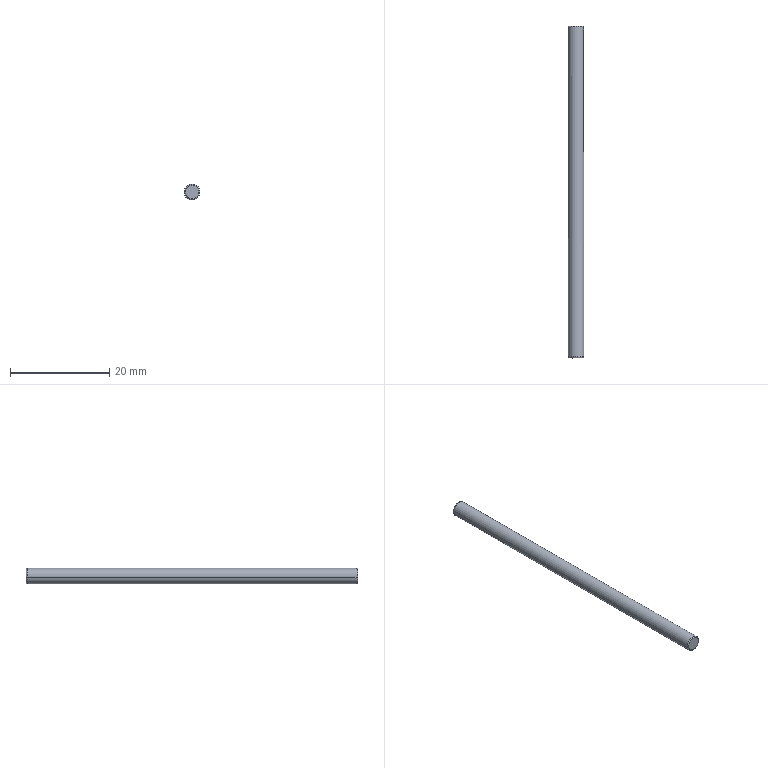Part | SolidWorks | features BaseBody 1 | 1 solid | 8 faces | box 3.204 x 67.003 x 3.14 mm | volume 518.664 mm3 | torus 4 | cylinder 2 | plane 2 | commonest cylinder face diameters 3.14 x2
STEP:
#1=CARTESIAN_POINT('',(340.446,372.663,106.551));
#2=VERTEX_POINT('',#1);
#3=CARTESIAN_POINT('',(343.498,372.666,107.288));
#4=VERTEX_POINT('',#3);
#5=CARTESIAN_POINT('',(341.972,372.664,106.919));
#6=DIRECTION('',(0.0009599,-1.,0.));
#7=DIRECTION('',(0.9721,0.0009331,0.2347));
#8=AXIS2_PLACEMENT_3D('',#5,#6,#7);
#9=CIRCLE('',#8,1.57);
#10=EDGE_CURVE('',#2,#4,#9,.T.);
#11=ORIENTED_EDGE('',*,*,#10,.T.);
#12=CARTESIAN_POINT('',(343.304,372.465,107.241));
#13=VERTEX_POINT('',#12);
#14=CARTESIAN_POINT('',(343.304,372.665,107.241));
#15=DIRECTION('',(0.2347,0.0002252,-0.9721));
#16=DIRECTION('',(-0.9721,0.,-0.2347));
#17=AXIS2_PLACEMENT_3D('',#14,#15,#16);
#18=CIRCLE('',#17,0.2);
#19=EDGE_CURVE('',#4,#13,#18,.T.);
#20=ORIENTED_EDGE('',*,*,#19,.T.);
#21=CARTESIAN_POINT('',(340.641,372.463,106.598));
#22=VERTEX_POINT('',#21);
#23=CARTESIAN_POINT('',(341.972,372.464,106.919));
#24=DIRECTION('',(0.0009599,-1.,0.));
#25=DIRECTION('',(0.9721,0.0009331,0.2347));
#26=AXIS2_PLACEMENT_3D('',#23,#24,#25);
#27=CIRCLE('',#26,1.37);
#28=EDGE_CURVE('',#22,#13,#27,.T.);
#29=ORIENTED_EDGE('',*,*,#28,.F.);
#30=CARTESIAN_POINT('',(340.64,372.663,106.598));
#31=DIRECTION('',(-0.2347,-0.0002252,0.9721));
#32=DIRECTION('',(0.9721,0.,0.2347));
#33=AXIS2_PLACEMENT_3D('',#30,#31,#32);
#34=CIRCLE('',#33,0.2);
#35=EDGE_CURVE('',#2,#22,#34,.T.);
#36=ORIENTED_EDGE('',*,*,#35,.F.);
#37=EDGE_LOOP('',(#11,#20,#29,#36));
#38=FACE_OUTER_BOUND('',#37,.T.);
#39=CARTESIAN_POINT('',(341.972,372.664,106.919));
#40=DIRECTION('',(0.0009599,-1.,0.));
#41=DIRECTION('',(-0.9721,-0.0009331,-0.2347));
#42=AXIS2_PLACEMENT_3D('',#39,#40,#41);
#43=TOROIDAL_SURFACE('',#42,1.37,0.2);
#44=ADVANCED_FACE('',(#38),#43,.T.);
#45=CARTESIAN_POINT('',(343.434,439.265,107.288));
#46=VERTEX_POINT('',#45);
#47=CARTESIAN_POINT('',(340.382,439.263,106.551));
#48=VERTEX_POINT('',#47);
#49=CARTESIAN_POINT('',(341.908,439.264,106.919));
#50=DIRECTION('',(-0.0009599,1.,0.));
#51=DIRECTION('',(0.9721,0.0009331,0.2347));
#52=AXIS2_PLACEMENT_3D('',#49,#50,#51);
#53=CIRCLE('',#52,1.57);
#54=EDGE_CURVE('',#46,#48,#53,.T.);
#55=ORIENTED_EDGE('',*,*,#54,.F.);
#56=CARTESIAN_POINT('',(343.434,439.465,107.288));
#57=DIRECTION('',(0.0009599,-1.,0.));
#58=VECTOR('',#57,1000.);
#59=LINE('',#56,#58);
#60=EDGE_CURVE('',#46,#4,#59,.T.);
#61=ORIENTED_EDGE('',*,*,#60,.T.);
#62=ORIENTED_EDGE('',*,*,#10,.F.);
#63=CARTESIAN_POINT('',(340.382,439.463,106.551));
#64=DIRECTION('',(0.0009599,-1.,0.));
#65=VECTOR('',#64,1000.);
#66=LINE('',#63,#65);
#67=EDGE_CURVE('',#48,#2,#66,.T.);
#68=ORIENTED_EDGE('',*,*,#67,.F.);
#69=EDGE_LOOP('',(#55,#61,#62,#68));
#70=FACE_OUTER_BOUND('',#69,.T.);
#71=CARTESIAN_POINT('',(341.908,439.464,106.919));
#72=DIRECTION('',(0.0009599,-1.,0.));
#73=DIRECTION('',(-0.9721,-0.0009331,-0.2347));
#74=AXIS2_PLACEMENT_3D('',#71,#72,#73);
#75=CYLINDRICAL_SURFACE('',#74,1.57);
#76=ADVANCED_FACE('',(#70),#75,.T.);
#77=CARTESIAN_POINT('',(343.24,439.465,107.241));
#78=VERTEX_POINT('',#77);
#79=CARTESIAN_POINT('',(340.576,439.463,106.598));
#80=VERTEX_POINT('',#79);
#81=CARTESIAN_POINT('',(341.908,439.464,106.919));
#82=DIRECTION('',(-0.0009599,1.,0.));
#83=DIRECTION('',(0.9721,0.0009331,0.2347));
#84=AXIS2_PLACEMENT_3D('',#81,#82,#83);
#85=CIRCLE('',#84,1.37);
#86=EDGE_CURVE('',#78,#80,#85,.T.);
#87=ORIENTED_EDGE('',*,*,#86,.F.);
#88=CARTESIAN_POINT('',(343.24,439.265,107.241));
#89=DIRECTION('',(0.2347,0.0002252,-0.9721));
#90=DIRECTION('',(-0.9721,0.,-0.2347));
#91=AXIS2_PLACEMENT_3D('',#88,#89,#90);
#92=CIRCLE('',#91,0.2);
#93=EDGE_CURVE('',#78,#46,#92,.T.);
#94=ORIENTED_EDGE('',*,*,#93,.T.);
#95=ORIENTED_EDGE('',*,*,#54,.T.);
#96=CARTESIAN_POINT('',(340.577,439.263,106.598));
#97=DIRECTION('',(-0.2347,-0.0002252,0.9721));
#98=DIRECTION('',(0.9721,0.,0.2347));
#99=AXIS2_PLACEMENT_3D('',#96,#97,#98);
#100=CIRCLE('',#99,0.2);
#101=EDGE_CURVE('',#80,#48,#100,.T.);
#102=ORIENTED_EDGE('',*,*,#101,.F.);
#103=EDGE_LOOP('',(#87,#94,#95,#102));
#104=FACE_OUTER_BOUND('',#103,.T.);
#105=CARTESIAN_POINT('',(341.908,439.264,106.919));
#106=DIRECTION('',(0.0009599,-1.,0.));
#107=DIRECTION('',(-0.9721,-0.0009331,-0.2347));
#108=AXIS2_PLACEMENT_3D('',#105,#106,#107);
#109=TOROIDAL_SURFACE('',#108,1.37,0.2);
#110=ADVANCED_FACE('',(#104),#109,.T.);
#111=ORIENTED_EDGE('',*,*,#28,.T.);
#112=CARTESIAN_POINT('',(341.972,372.464,106.919));
#113=DIRECTION('',(0.0009599,-1.,0.));
#114=DIRECTION('',(0.9721,0.0009331,0.2347));
#115=AXIS2_PLACEMENT_3D('',#112,#113,#114);
#116=CIRCLE('',#115,1.37);
#117=EDGE_CURVE('',#13,#22,#116,.T.);
#118=ORIENTED_EDGE('',*,*,#117,.T.);
#119=EDGE_LOOP('',(#111,#118));
#120=FACE_OUTER_BOUND('',#119,.T.);
#121=CARTESIAN_POINT('',(341.972,372.464,106.919));
#122=DIRECTION('',(0.0009599,-1.,0.));
#123=DIRECTION('',(0.,0.,-1.));
#124=AXIS2_PLACEMENT_3D('',#121,#122,#123);
#125=PLANE('',#124);
#126=ADVANCED_FACE('',(#120),#125,.T.);
#127=CARTESIAN_POINT('',(341.908,439.464,106.919));
#128=DIRECTION('',(-0.0009599,1.,0.));
#129=DIRECTION('',(0.9721,0.0009331,0.2347));
#130=AXIS2_PLACEMENT_3D('',#127,#128,#129);
#131=CIRCLE('',#130,1.37);
#132=EDGE_CURVE('',#80,#78,#131,.T.);
#133=ORIENTED_EDGE('',*,*,#132,.T.);
#134=ORIENTED_EDGE('',*,*,#86,.T.);
#135=EDGE_LOOP('',(#133,#134));
#136=FACE_OUTER_BOUND('',#135,.T.);
#137=CARTESIAN_POINT('',(341.908,439.464,106.919));
#138=DIRECTION('',(0.0009599,-1.,0.));
#139=DIRECTION('',(0.,0.,-1.));
#140=AXIS2_PLACEMENT_3D('',#137,#138,#139);
#141=PLANE('',#140);
#142=ADVANCED_FACE('',(#136),#141,.F.);
#143=ORIENTED_EDGE('',*,*,#93,.F.);
#144=ORIENTED_EDGE('',*,*,#132,.F.);
#145=ORIENTED_EDGE('',*,*,#101,.T.);
#146=CARTESIAN_POINT('',(341.908,439.264,106.919));
#147=DIRECTION('',(-0.0009599,1.,0.));
#148=DIRECTION('',(0.9721,0.0009331,0.2347));
#149=AXIS2_PLACEMENT_3D('',#146,#147,#148);
#150=CIRCLE('',#149,1.57);
#151=EDGE_CURVE('',#48,#46,#150,.T.);
#152=ORIENTED_EDGE('',*,*,#151,.T.);
#153=EDGE_LOOP('',(#143,#144,#145,#152));
#154=FACE_OUTER_BOUND('',#153,.T.);
#155=CARTESIAN_POINT('',(341.908,439.264,106.919));
#156=DIRECTION('',(0.0009599,-1.,0.));
#157=DIRECTION('',(-0.9721,-0.0009331,-0.2347));
#158=AXIS2_PLACEMENT_3D('',#155,#156,#157);
#159=TOROIDAL_SURFACE('',#158,1.37,0.2);
#160=ADVANCED_FACE('',(#154),#159,.T.);
#161=ORIENTED_EDGE('',*,*,#60,.F.);
#162=ORIENTED_EDGE('',*,*,#151,.F.);
#163=ORIENTED_EDGE('',*,*,#67,.T.);
#164=CARTESIAN_POINT('',(341.972,372.664,106.919));
#165=DIRECTION('',(0.0009599,-1.,0.));
#166=DIRECTION('',(0.9721,0.0009331,0.2347));
#167=AXIS2_PLACEMENT_3D('',#164,#165,#166);
#168=CIRCLE('',#167,1.57);
#169=EDGE_CURVE('',#4,#2,#168,.T.);
#170=ORIENTED_EDGE('',*,*,#169,.F.);
#171=EDGE_LOOP('',(#161,#162,#163,#170));
#172=FACE_OUTER_BOUND('',#171,.T.);
#173=CARTESIAN_POINT('',(341.908,439.464,106.919));
#174=DIRECTION('',(0.0009599,-1.,0.));
#175=DIRECTION('',(-0.9721,-0.0009331,-0.2347));
#176=AXIS2_PLACEMENT_3D('',#173,#174,#175);
#177=CYLINDRICAL_SURFACE('',#176,1.57);
#178=ADVANCED_FACE('',(#172),#177,.T.);
#179=ORIENTED_EDGE('',*,*,#19,.F.);
#180=ORIENTED_EDGE('',*,*,#169,.T.);
#181=ORIENTED_EDGE('',*,*,#35,.T.);
#182=ORIENTED_EDGE('',*,*,#117,.F.);
#183=EDGE_LOOP('',(#179,#180,#181,#182));
#184=FACE_OUTER_BOUND('',#183,.T.);
#185=CARTESIAN_POINT('',(341.972,372.664,106.919));
#186=DIRECTION('',(0.0009599,-1.,0.));
#187=DIRECTION('',(-0.9721,-0.0009331,-0.2347));
#188=AXIS2_PLACEMENT_3D('',#185,#186,#187);
#189=TOROIDAL_SURFACE('',#188,1.37,0.2);
#190=ADVANCED_FACE('',(#184),#189,.T.);
#191=CLOSED_SHELL('',(#44,#76,#110,#126,#142,#160,#178,#190));
#192=MANIFOLD_SOLID_BREP('',#191);
#193=CARTESIAN_POINT('',(0.,0.,0.));
#194=DIRECTION('',(0.,0.,1.));
#195=DIRECTION('',(1.,0.,0.));
#196=AXIS2_PLACEMENT_3D('',#193,#194,#195);
#197=(LENGTH_UNIT()NAMED_UNIT(*)SI_UNIT(.MILLI.,.METRE.));
#198=UNCERTAINTY_MEASURE_WITH_UNIT(LENGTH_MEASURE(0.00001),#197,'','');
#199=(NAMED_UNIT(*)PLANE_ANGLE_UNIT()SI_UNIT($,.RADIAN.));
#200=(NAMED_UNIT(*)SI_UNIT($,.STERADIAN.)SOLID_ANGLE_UNIT());
#201=(GEOMETRIC_REPRESENTATION_CONTEXT(3)GLOBAL_UNCERTAINTY_ASSIGNED_CONTEXT((#198))GLOBAL_UNIT_ASSIGNED_CONTEXT((#197,#199,#200))REPRESENTATION_CONTEXT('',''));
#202=ADVANCED_BREP_SHAPE_REPRESENTATION('',(#192,#196),#201);